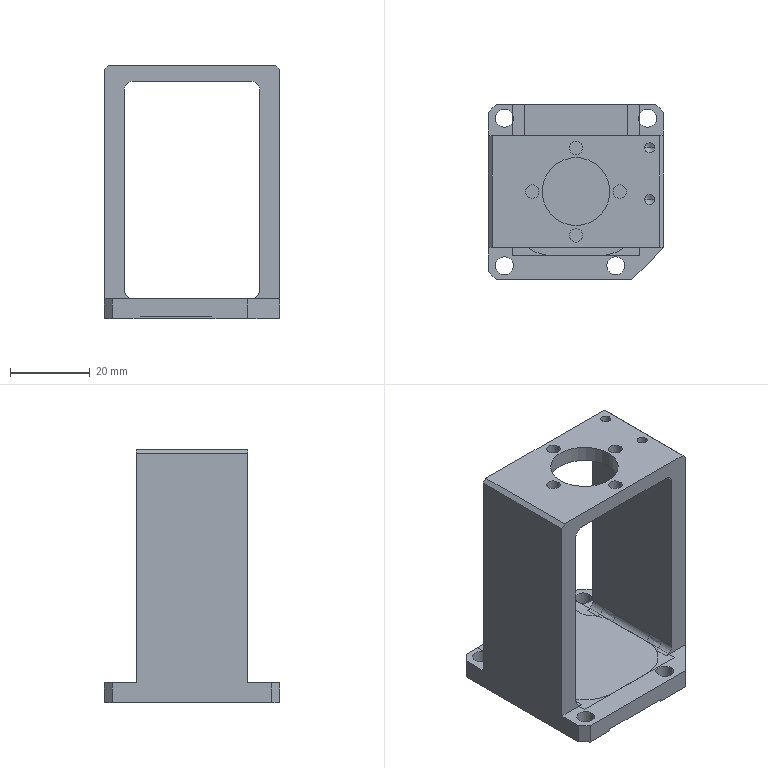Part | 2 solids | 78 faces | box 44 x 44 x 63.6 mm | volume 28804 mm3 | plane 36 | cylinder 34 | cone 4 | spline 4 | commonest cylinder face diameters 3.4 x8 4 x8 4.5 x8 2.5 x4 20 x4 17 x2